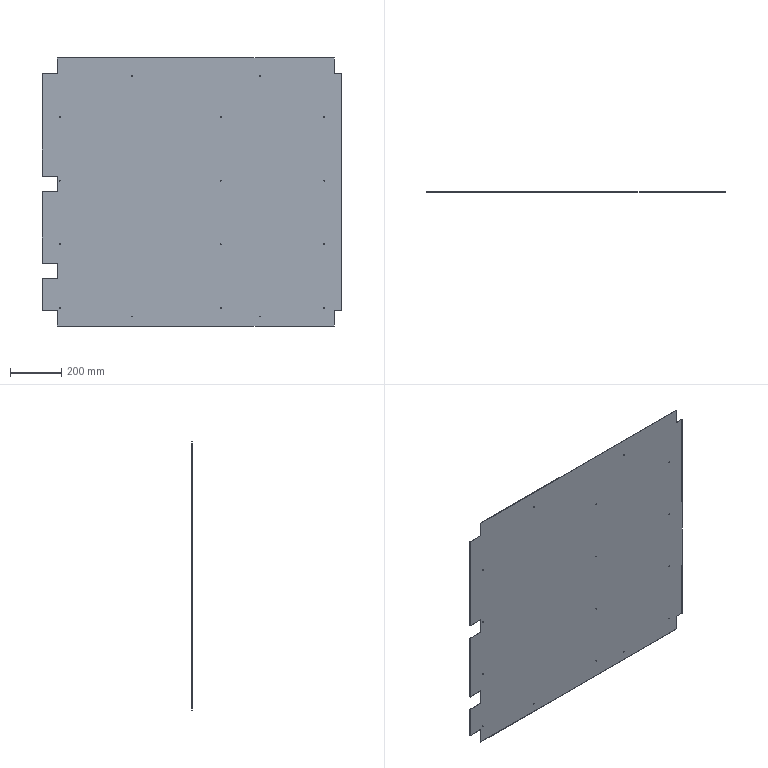Part | NX | features BREP 1 | 1 solid | 54 faces | box 1175 x 1.5 x 1050 mm | volume 1824301 mm3 | cylinder 32 | plane 22 | commonest cylinder face diameters 3.3 x32